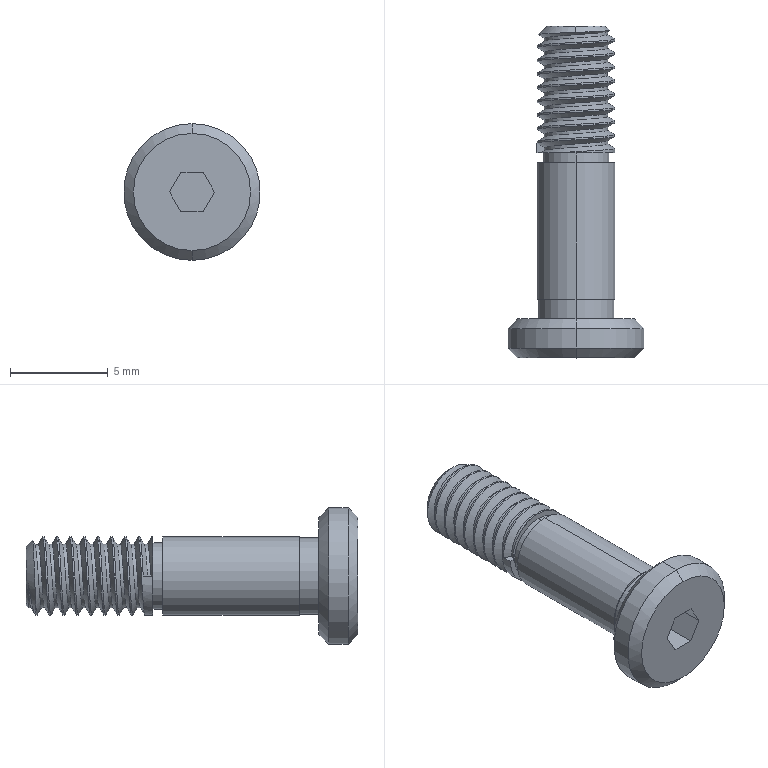Part | NX | features BREP 1 | 1 solid | 51 faces | box 7 x 17 x 7 mm | volume 233.928 mm3 | cylinder 28 | plane 14 | cone 7 | spline 2 | commonest cylinder face diameters 4 x21 3.4 x2 3.9 x2 7 x2 3.242 x1